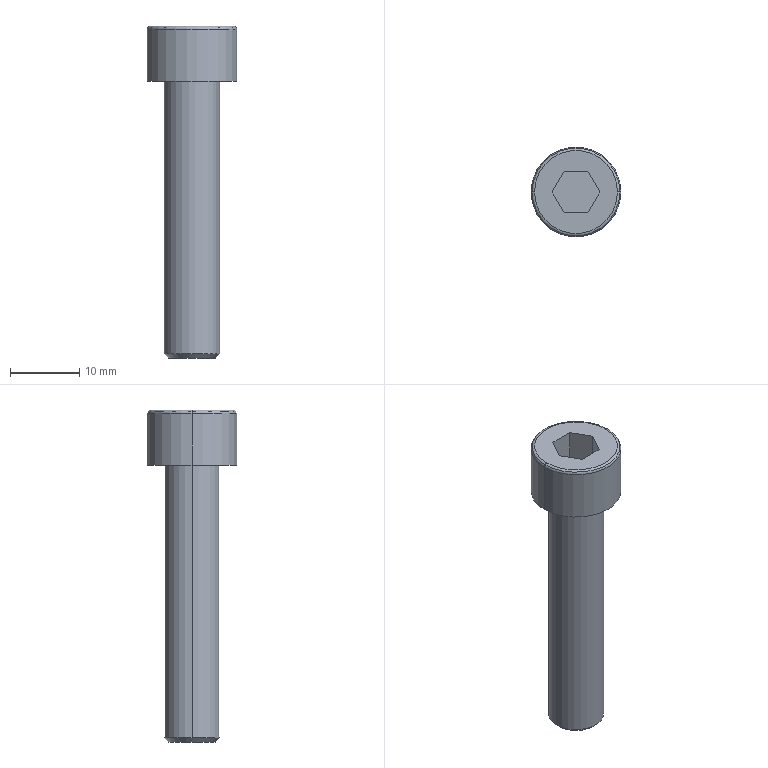Part | Creo | 1 solid | 20 faces | box 13 x 13 x 48 mm | volume 2901 mm3 | plane 10 | torus 4 | cylinder 4 | cone 2 | commonest cylinder face diameters 8 x2 13 x2
STEP:
#1=CARTESIAN_POINT('',(143.362,-96.002,37.161));
#2=VERTEX_POINT('',#1);
#3=CARTESIAN_POINT('',(131.362,-96.002,37.161));
#4=VERTEX_POINT('',#3);
#5=CARTESIAN_POINT('',(137.362,-96.002,37.161));
#6=DIRECTION('',(0.,0.,1.));
#7=DIRECTION('',(1.,0.,0.));
#8=AXIS2_PLACEMENT_3D('',#5,#6,#7);
#9=CIRCLE('',#8,6.);
#10=EDGE_CURVE('',#2,#4,#9,.T.);
#11=ORIENTED_EDGE('',*,*,#10,.F.);
#12=CARTESIAN_POINT('',(137.362,-96.002,37.161));
#13=DIRECTION('',(0.,0.,1.));
#14=DIRECTION('',(-1.,0.,0.));
#15=AXIS2_PLACEMENT_3D('',#12,#13,#14);
#16=CIRCLE('',#15,6.);
#17=EDGE_CURVE('',#4,#2,#16,.T.);
#18=ORIENTED_EDGE('',*,*,#17,.F.);
#19=EDGE_LOOP('',(#11,#18));
#20=FACE_OUTER_BOUND('',#19,.F.);
#21=CARTESIAN_POINT('',(139.094,-93.002,37.161));
#22=VERTEX_POINT('',#21);
#23=CARTESIAN_POINT('',(135.63,-93.002,37.161));
#24=VERTEX_POINT('',#23);
#25=CARTESIAN_POINT('',(139.094,-93.002,37.161));
#26=DIRECTION('',(-1.,0.,0.));
#27=VECTOR('',#26,3.464);
#28=LINE('',#25,#27);
#29=EDGE_CURVE('',#22,#24,#28,.T.);
#30=ORIENTED_EDGE('',*,*,#29,.T.);
#31=CARTESIAN_POINT('',(133.898,-96.002,37.161));
#32=VERTEX_POINT('',#31);
#33=CARTESIAN_POINT('',(133.898,-96.002,37.161));
#34=DIRECTION('',(0.5,0.866,0.));
#35=VECTOR('',#34,3.464);
#36=LINE('',#33,#35);
#37=EDGE_CURVE('',#32,#24,#36,.T.);
#38=ORIENTED_EDGE('',*,*,#37,.F.);
#39=CARTESIAN_POINT('',(135.63,-99.002,37.161));
#40=VERTEX_POINT('',#39);
#41=CARTESIAN_POINT('',(135.63,-99.002,37.161));
#42=DIRECTION('',(-0.5,0.866,0.));
#43=VECTOR('',#42,3.464);
#44=LINE('',#41,#43);
#45=EDGE_CURVE('',#40,#32,#44,.T.);
#46=ORIENTED_EDGE('',*,*,#45,.F.);
#47=CARTESIAN_POINT('',(139.094,-99.002,37.161));
#48=VERTEX_POINT('',#47);
#49=CARTESIAN_POINT('',(135.63,-99.002,37.161));
#50=DIRECTION('',(1.,0.,0.));
#51=VECTOR('',#50,3.464);
#52=LINE('',#49,#51);
#53=EDGE_CURVE('',#40,#48,#52,.T.);
#54=ORIENTED_EDGE('',*,*,#53,.T.);
#55=CARTESIAN_POINT('',(140.826,-96.002,37.161));
#56=VERTEX_POINT('',#55);
#57=CARTESIAN_POINT('',(140.826,-96.002,37.161));
#58=DIRECTION('',(-0.5,-0.866,0.));
#59=VECTOR('',#58,3.464);
#60=LINE('',#57,#59);
#61=EDGE_CURVE('',#56,#48,#60,.T.);
#62=ORIENTED_EDGE('',*,*,#61,.F.);
#63=CARTESIAN_POINT('',(139.094,-93.002,37.161));
#64=DIRECTION('',(0.5,-0.866,0.));
#65=VECTOR('',#64,3.464);
#66=LINE('',#63,#65);
#67=EDGE_CURVE('',#22,#56,#66,.T.);
#68=ORIENTED_EDGE('',*,*,#67,.F.);
#69=EDGE_LOOP('',(#30,#38,#46,#54,#62,#68));
#70=FACE_BOUND('',#69,.F.);
#71=CARTESIAN_POINT('',(137.362,-96.002,37.161));
#72=DIRECTION('',(0.,0.,1.));
#73=DIRECTION('',(1.,0.,0.));
#74=AXIS2_PLACEMENT_3D('',#71,#72,#73);
#75=PLANE('',#74);
#76=ADVANCED_FACE('',(#20,#70),#75,.T.);
#77=ORIENTED_EDGE('',*,*,#10,.T.);
#78=CARTESIAN_POINT('',(131.008,-96.002,37.014));
#79=VERTEX_POINT('',#78);
#80=CARTESIAN_POINT('',(131.362,-96.002,36.661));
#81=DIRECTION('',(0.,1.,0.));
#82=DIRECTION('',(-0.7071,0.,0.7071));
#83=AXIS2_PLACEMENT_3D('',#80,#81,#82);
#84=CIRCLE('',#83,0.5);
#85=EDGE_CURVE('',#79,#4,#84,.T.);
#86=ORIENTED_EDGE('',*,*,#85,.F.);
#87=CARTESIAN_POINT('',(143.715,-96.002,37.014));
#88=VERTEX_POINT('',#87);
#89=CARTESIAN_POINT('',(137.362,-96.002,37.014));
#90=DIRECTION('',(0.,0.,1.));
#91=DIRECTION('',(1.,0.,0.));
#92=AXIS2_PLACEMENT_3D('',#89,#90,#91);
#93=CIRCLE('',#92,6.354);
#94=EDGE_CURVE('',#88,#79,#93,.T.);
#95=ORIENTED_EDGE('',*,*,#94,.F.);
#96=CARTESIAN_POINT('',(143.362,-96.002,36.661));
#97=DIRECTION('',(0.,-1.,0.));
#98=DIRECTION('',(0.7071,0.,0.7071));
#99=AXIS2_PLACEMENT_3D('',#96,#97,#98);
#100=CIRCLE('',#99,0.5);
#101=EDGE_CURVE('',#88,#2,#100,.T.);
#102=ORIENTED_EDGE('',*,*,#101,.T.);
#103=EDGE_LOOP('',(#77,#86,#95,#102));
#104=FACE_OUTER_BOUND('',#103,.F.);
#105=CARTESIAN_POINT('',(137.362,-96.002,36.661));
#106=DIRECTION('',(0.,0.,1.));
#107=DIRECTION('',(1.,0.,0.));
#108=AXIS2_PLACEMENT_3D('',#105,#106,#107);
#109=TOROIDAL_SURFACE('',#108,6.,0.5);
#110=ADVANCED_FACE('',(#104),#109,.T.);
#111=ORIENTED_EDGE('',*,*,#17,.T.);
#112=ORIENTED_EDGE('',*,*,#101,.F.);
#113=CARTESIAN_POINT('',(137.362,-96.002,37.014));
#114=DIRECTION('',(0.,0.,1.));
#115=DIRECTION('',(-1.,0.,0.));
#116=AXIS2_PLACEMENT_3D('',#113,#114,#115);
#117=CIRCLE('',#116,6.354);
#118=EDGE_CURVE('',#79,#88,#117,.T.);
#119=ORIENTED_EDGE('',*,*,#118,.F.);
#120=ORIENTED_EDGE('',*,*,#85,.T.);
#121=EDGE_LOOP('',(#111,#112,#119,#120));
#122=FACE_OUTER_BOUND('',#121,.F.);
#123=CARTESIAN_POINT('',(137.362,-96.002,36.661));
#124=DIRECTION('',(0.,0.,1.));
#125=DIRECTION('',(1.,0.,0.));
#126=AXIS2_PLACEMENT_3D('',#123,#124,#125);
#127=TOROIDAL_SURFACE('',#126,6.,0.5);
#128=ADVANCED_FACE('',(#122),#127,.T.);
#129=CARTESIAN_POINT('',(130.862,-96.002,36.661));
#130=VERTEX_POINT('',#129);
#131=CARTESIAN_POINT('',(143.862,-96.002,36.661));
#132=VERTEX_POINT('',#131);
#133=CARTESIAN_POINT('',(137.362,-96.002,36.661));
#134=DIRECTION('',(0.,0.,1.));
#135=DIRECTION('',(-1.,0.,0.));
#136=AXIS2_PLACEMENT_3D('',#133,#134,#135);
#137=CIRCLE('',#136,6.5);
#138=EDGE_CURVE('',#130,#132,#137,.T.);
#139=ORIENTED_EDGE('',*,*,#138,.F.);
#140=CARTESIAN_POINT('',(131.362,-96.002,36.661));
#141=DIRECTION('',(0.,1.,0.));
#142=DIRECTION('',(-1.,0.,0.));
#143=AXIS2_PLACEMENT_3D('',#140,#141,#142);
#144=CIRCLE('',#143,0.5);
#145=EDGE_CURVE('',#130,#79,#144,.T.);
#146=ORIENTED_EDGE('',*,*,#145,.T.);
#147=ORIENTED_EDGE('',*,*,#118,.T.);
#148=CARTESIAN_POINT('',(143.362,-96.002,36.661));
#149=DIRECTION('',(0.,-1.,0.));
#150=DIRECTION('',(1.,0.,0.));
#151=AXIS2_PLACEMENT_3D('',#148,#149,#150);
#152=CIRCLE('',#151,0.5);
#153=EDGE_CURVE('',#132,#88,#152,.T.);
#154=ORIENTED_EDGE('',*,*,#153,.F.);
#155=EDGE_LOOP('',(#139,#146,#147,#154));
#156=FACE_OUTER_BOUND('',#155,.F.);
#157=CARTESIAN_POINT('',(137.362,-96.002,36.661));
#158=DIRECTION('',(0.,0.,1.));
#159=DIRECTION('',(1.,0.,0.));
#160=AXIS2_PLACEMENT_3D('',#157,#158,#159);
#161=TOROIDAL_SURFACE('',#160,6.,0.5);
#162=ADVANCED_FACE('',(#156),#161,.T.);
#163=ORIENTED_EDGE('',*,*,#138,.T.);
#164=CARTESIAN_POINT('',(143.862,-96.002,29.161));
#165=VERTEX_POINT('',#164);
#166=CARTESIAN_POINT('',(143.862,-96.002,29.161));
#167=DIRECTION('',(0.,0.,1.));
#168=VECTOR('',#167,7.5);
#169=LINE('',#166,#168);
#170=EDGE_CURVE('',#165,#132,#169,.T.);
#171=ORIENTED_EDGE('',*,*,#170,.F.);
#172=CARTESIAN_POINT('',(130.862,-96.002,29.161));
#173=VERTEX_POINT('',#172);
#174=CARTESIAN_POINT('',(137.362,-96.002,29.161));
#175=DIRECTION('',(0.,0.,-1.));
#176=DIRECTION('',(1.,0.,0.));
#177=AXIS2_PLACEMENT_3D('',#174,#175,#176);
#178=CIRCLE('',#177,6.5);
#179=EDGE_CURVE('',#165,#173,#178,.T.);
#180=ORIENTED_EDGE('',*,*,#179,.T.);
#181=CARTESIAN_POINT('',(130.862,-96.002,29.161));
#182=DIRECTION('',(0.,0.,1.));
#183=VECTOR('',#182,7.5);
#184=LINE('',#181,#183);
#185=EDGE_CURVE('',#173,#130,#184,.T.);
#186=ORIENTED_EDGE('',*,*,#185,.T.);
#187=EDGE_LOOP('',(#163,#171,#180,#186));
#188=FACE_OUTER_BOUND('',#187,.F.);
#189=CARTESIAN_POINT('',(137.362,-96.002,29.161));
#190=DIRECTION('',(0.,0.,1.));
#191=DIRECTION('',(1.,0.,0.));
#192=AXIS2_PLACEMENT_3D('',#189,#190,#191);
#193=CYLINDRICAL_SURFACE('',#192,6.5);
#194=ADVANCED_FACE('',(#188),#193,.T.);
#195=CARTESIAN_POINT('',(137.362,-96.002,36.661));
#196=DIRECTION('',(0.,0.,1.));
#197=DIRECTION('',(1.,0.,0.));
#198=AXIS2_PLACEMENT_3D('',#195,#196,#197);
#199=CIRCLE('',#198,6.5);
#200=EDGE_CURVE('',#132,#130,#199,.T.);
#201=ORIENTED_EDGE('',*,*,#200,.T.);
#202=ORIENTED_EDGE('',*,*,#185,.F.);
#203=CARTESIAN_POINT('',(137.362,-96.002,29.161));
#204=DIRECTION('',(0.,0.,-1.));
#205=DIRECTION('',(-1.,0.,0.));
#206=AXIS2_PLACEMENT_3D('',#203,#204,#205);
#207=CIRCLE('',#206,6.5);
#208=EDGE_CURVE('',#173,#165,#207,.T.);
#209=ORIENTED_EDGE('',*,*,#208,.T.);
#210=ORIENTED_EDGE('',*,*,#170,.T.);
#211=EDGE_LOOP('',(#201,#202,#209,#210));
#212=FACE_OUTER_BOUND('',#211,.F.);
#213=CARTESIAN_POINT('',(137.362,-96.002,29.161));
#214=DIRECTION('',(0.,0.,1.));
#215=DIRECTION('',(1.,0.,0.));
#216=AXIS2_PLACEMENT_3D('',#213,#214,#215);
#217=CYLINDRICAL_SURFACE('',#216,6.5);
#218=ADVANCED_FACE('',(#212),#217,.T.);
#219=ORIENTED_EDGE('',*,*,#200,.F.);
#220=ORIENTED_EDGE('',*,*,#153,.T.);
#221=ORIENTED_EDGE('',*,*,#94,.T.);
#222=ORIENTED_EDGE('',*,*,#145,.F.);
#223=EDGE_LOOP('',(#219,#220,#221,#222));
#224=FACE_OUTER_BOUND('',#223,.F.);
#225=CARTESIAN_POINT('',(137.362,-96.002,36.661));
#226=DIRECTION('',(0.,0.,1.));
#227=DIRECTION('',(1.,0.,0.));
#228=AXIS2_PLACEMENT_3D('',#225,#226,#227);
#229=TOROIDAL_SURFACE('',#228,6.,0.5);
#230=ADVANCED_FACE('',(#224),#229,.T.);
#231=ORIENTED_EDGE('',*,*,#179,.F.);
#232=ORIENTED_EDGE('',*,*,#208,.F.);
#233=EDGE_LOOP('',(#231,#232));
#234=FACE_OUTER_BOUND('',#233,.F.);
#235=CARTESIAN_POINT('',(141.362,-96.002,29.161));
#236=VERTEX_POINT('',#235);
#237=CARTESIAN_POINT('',(133.362,-96.002,29.161));
#238=VERTEX_POINT('',#237);
#239=CARTESIAN_POINT('',(137.362,-96.002,29.161));
#240=DIRECTION('',(0.,0.,1.));
#241=DIRECTION('',(1.,0.,0.));
#242=AXIS2_PLACEMENT_3D('',#239,#240,#241);
#243=CIRCLE('',#242,4.);
#244=EDGE_CURVE('',#236,#238,#243,.T.);
#245=ORIENTED_EDGE('',*,*,#244,.F.);
#246=CARTESIAN_POINT('',(137.362,-96.002,29.161));
#247=DIRECTION('',(0.,0.,1.));
#248=DIRECTION('',(-1.,0.,0.));
#249=AXIS2_PLACEMENT_3D('',#246,#247,#248);
#250=CIRCLE('',#249,4.);
#251=EDGE_CURVE('',#238,#236,#250,.T.);
#252=ORIENTED_EDGE('',*,*,#251,.F.);
#253=EDGE_LOOP('',(#245,#252));
#254=FACE_BOUND('',#253,.F.);
#255=CARTESIAN_POINT('',(137.362,-96.002,29.161));
#256=DIRECTION('',(0.,0.,-1.));
#257=DIRECTION('',(-1.,0.,0.));
#258=AXIS2_PLACEMENT_3D('',#255,#256,#257);
#259=PLANE('',#258);
#260=ADVANCED_FACE('',(#234,#254),#259,.T.);
#261=CARTESIAN_POINT('',(133.362,-96.002,-10.239));
#262=VERTEX_POINT('',#261);
#263=CARTESIAN_POINT('',(141.362,-96.002,-10.239));
#264=VERTEX_POINT('',#263);
#265=CARTESIAN_POINT('',(137.362,-96.002,-10.239));
#266=DIRECTION('',(0.,0.,-1.));
#267=DIRECTION('',(-1.,0.,0.));
#268=AXIS2_PLACEMENT_3D('',#265,#266,#267);
#269=CIRCLE('',#268,4.);
#270=EDGE_CURVE('',#262,#264,#269,.T.);
#271=ORIENTED_EDGE('',*,*,#270,.T.);
#272=CARTESIAN_POINT('',(141.362,-96.002,-10.239));
#273=DIRECTION('',(0.,0.,1.));
#274=VECTOR('',#273,39.4);
#275=LINE('',#272,#274);
#276=EDGE_CURVE('',#264,#236,#275,.T.);
#277=ORIENTED_EDGE('',*,*,#276,.T.);
#278=ORIENTED_EDGE('',*,*,#244,.T.);
#279=CARTESIAN_POINT('',(133.362,-96.002,-10.239));
#280=DIRECTION('',(0.,0.,1.));
#281=VECTOR('',#280,39.4);
#282=LINE('',#279,#281);
#283=EDGE_CURVE('',#262,#238,#282,.T.);
#284=ORIENTED_EDGE('',*,*,#283,.F.);
#285=EDGE_LOOP('',(#271,#277,#278,#284));
#286=FACE_OUTER_BOUND('',#285,.F.);
#287=CARTESIAN_POINT('',(137.362,-96.002,-10.839));
#288=DIRECTION('',(0.,0.,1.));
#289=DIRECTION('',(1.,0.,0.));
#290=AXIS2_PLACEMENT_3D('',#287,#288,#289);
#291=CYLINDRICAL_SURFACE('',#290,4.);
#292=ADVANCED_FACE('',(#286),#291,.T.);
#293=CARTESIAN_POINT('',(133.962,-96.002,-10.839));
#294=VERTEX_POINT('',#293);
#295=CARTESIAN_POINT('',(140.762,-96.002,-10.839));
#296=VERTEX_POINT('',#295);
#297=CARTESIAN_POINT('',(137.362,-96.002,-10.839));
#298=DIRECTION('',(0.,0.,-1.));
#299=DIRECTION('',(-1.,0.,0.));
#300=AXIS2_PLACEMENT_3D('',#297,#298,#299);
#301=CIRCLE('',#300,3.4);
#302=EDGE_CURVE('',#294,#296,#301,.T.);
#303=ORIENTED_EDGE('',*,*,#302,.T.);
#304=CARTESIAN_POINT('',(140.762,-96.002,-10.839));
#305=DIRECTION('',(0.7071,0.,0.7071));
#306=VECTOR('',#305,0.8485);
#307=LINE('',#304,#306);
#308=EDGE_CURVE('',#296,#264,#307,.T.);
#309=ORIENTED_EDGE('',*,*,#308,.T.);
#310=ORIENTED_EDGE('',*,*,#270,.F.);
#311=CARTESIAN_POINT('',(133.962,-96.002,-10.839));
#312=DIRECTION('',(-0.7071,0.,0.7071));
#313=VECTOR('',#312,0.8485);
#314=LINE('',#311,#313);
#315=EDGE_CURVE('',#294,#262,#314,.T.);
#316=ORIENTED_EDGE('',*,*,#315,.F.);
#317=EDGE_LOOP('',(#303,#309,#310,#316));
#318=FACE_OUTER_BOUND('',#317,.F.);
#319=CARTESIAN_POINT('',(137.362,-96.002,-10.539));
#320=DIRECTION('',(0.,0.,1.));
#321=DIRECTION('',(1.,0.,0.));
#322=AXIS2_PLACEMENT_3D('',#319,#320,#321);
#323=CONICAL_SURFACE('',#322,3.7,45.);
#324=ADVANCED_FACE('',(#318),#323,.T.);
#325=CARTESIAN_POINT('',(137.362,-96.002,-10.839));
#326=DIRECTION('',(0.,0.,-1.));
#327=DIRECTION('',(1.,0.,0.));
#328=AXIS2_PLACEMENT_3D('',#325,#326,#327);
#329=CIRCLE('',#328,3.4);
#330=EDGE_CURVE('',#296,#294,#329,.T.);
#331=ORIENTED_EDGE('',*,*,#330,.F.);
#332=ORIENTED_EDGE('',*,*,#302,.F.);
#333=EDGE_LOOP('',(#331,#332));
#334=FACE_OUTER_BOUND('',#333,.F.);
#335=CARTESIAN_POINT('',(137.362,-96.002,-10.839));
#336=DIRECTION('',(0.,0.,1.));
#337=DIRECTION('',(1.,0.,0.));
#338=AXIS2_PLACEMENT_3D('',#335,#336,#337);
#339=PLANE('',#338);
#340=ADVANCED_FACE('',(#334),#339,.F.);
#341=ORIENTED_EDGE('',*,*,#330,.T.);
#342=ORIENTED_EDGE('',*,*,#315,.T.);
#343=CARTESIAN_POINT('',(137.362,-96.002,-10.239));
#344=DIRECTION('',(0.,0.,-1.));
#345=DIRECTION('',(1.,0.,0.));
#346=AXIS2_PLACEMENT_3D('',#343,#344,#345);
#347=CIRCLE('',#346,4.);
#348=EDGE_CURVE('',#264,#262,#347,.T.);
#349=ORIENTED_EDGE('',*,*,#348,.F.);
#350=ORIENTED_EDGE('',*,*,#308,.F.);
#351=EDGE_LOOP('',(#341,#342,#349,#350));
#352=FACE_OUTER_BOUND('',#351,.F.);
#353=CARTESIAN_POINT('',(137.362,-96.002,-10.539));
#354=DIRECTION('',(0.,0.,1.));
#355=DIRECTION('',(1.,0.,0.));
#356=AXIS2_PLACEMENT_3D('',#353,#354,#355);
#357=CONICAL_SURFACE('',#356,3.7,45.);
#358=ADVANCED_FACE('',(#352),#357,.T.);
#359=ORIENTED_EDGE('',*,*,#348,.T.);
#360=ORIENTED_EDGE('',*,*,#283,.T.);
#361=ORIENTED_EDGE('',*,*,#251,.T.);
#362=ORIENTED_EDGE('',*,*,#276,.F.);
#363=EDGE_LOOP('',(#359,#360,#361,#362));
#364=FACE_OUTER_BOUND('',#363,.F.);
#365=CARTESIAN_POINT('',(137.362,-96.002,-10.839));
#366=DIRECTION('',(0.,0.,1.));
#367=DIRECTION('',(1.,0.,0.));
#368=AXIS2_PLACEMENT_3D('',#365,#366,#367);
#369=CYLINDRICAL_SURFACE('',#368,4.);
#370=ADVANCED_FACE('',(#364),#369,.T.);
#371=ORIENTED_EDGE('',*,*,#29,.F.);
#372=CARTESIAN_POINT('',(139.094,-93.002,31.881));
#373=VERTEX_POINT('',#372);
#374=CARTESIAN_POINT('',(139.094,-93.002,37.161));
#375=DIRECTION('',(0.,0.,-1.));
#376=VECTOR('',#375,5.28);
#377=LINE('',#374,#376);
#378=EDGE_CURVE('',#22,#373,#377,.T.);
#379=ORIENTED_EDGE('',*,*,#378,.T.);
#380=CARTESIAN_POINT('',(135.63,-93.002,31.881));
#381=VERTEX_POINT('',#380);
#382=CARTESIAN_POINT('',(139.094,-93.002,31.881));
#383=DIRECTION('',(-1.,0.,0.));
#384=VECTOR('',#383,3.464);
#385=LINE('',#382,#384);
#386=EDGE_CURVE('',#373,#381,#385,.T.);
#387=ORIENTED_EDGE('',*,*,#386,.T.);
#388=CARTESIAN_POINT('',(135.63,-93.002,37.161));
#389=DIRECTION('',(0.,0.,-1.));
#390=VECTOR('',#389,5.28);
#391=LINE('',#388,#390);
#392=EDGE_CURVE('',#24,#381,#391,.T.);
#393=ORIENTED_EDGE('',*,*,#392,.F.);
#394=EDGE_LOOP('',(#371,#379,#387,#393));
#395=FACE_OUTER_BOUND('',#394,.F.);
#396=CARTESIAN_POINT('',(135.63,-93.002,31.881));
#397=DIRECTION('',(0.,-1.,0.));
#398=DIRECTION('',(0.,0.,-1.));
#399=AXIS2_PLACEMENT_3D('',#396,#397,#398);
#400=PLANE('',#399);
#401=ADVANCED_FACE('',(#395),#400,.T.);
#402=ORIENTED_EDGE('',*,*,#67,.T.);
#403=CARTESIAN_POINT('',(140.826,-96.002,31.881));
#404=VERTEX_POINT('',#403);
#405=CARTESIAN_POINT('',(140.826,-96.002,37.161));
#406=DIRECTION('',(0.,0.,-1.));
#407=VECTOR('',#406,5.28);
#408=LINE('',#405,#407);
#409=EDGE_CURVE('',#56,#404,#408,.T.);
#410=ORIENTED_EDGE('',*,*,#409,.T.);
#411=CARTESIAN_POINT('',(140.826,-96.002,31.881));
#412=DIRECTION('',(-0.5,0.866,0.));
#413=VECTOR('',#412,3.464);
#414=LINE('',#411,#413);
#415=EDGE_CURVE('',#404,#373,#414,.T.);
#416=ORIENTED_EDGE('',*,*,#415,.T.);
#417=ORIENTED_EDGE('',*,*,#378,.F.);
#418=EDGE_LOOP('',(#402,#410,#416,#417));
#419=FACE_OUTER_BOUND('',#418,.F.);
#420=CARTESIAN_POINT('',(139.094,-93.002,31.881));
#421=DIRECTION('',(-0.866,-0.5,0.));
#422=DIRECTION('',(0.5,-0.866,0.));
#423=AXIS2_PLACEMENT_3D('',#420,#421,#422);
#424=PLANE('',#423);
#425=ADVANCED_FACE('',(#419),#424,.T.);
#426=ORIENTED_EDGE('',*,*,#61,.T.);
#427=CARTESIAN_POINT('',(139.094,-99.002,31.881));
#428=VERTEX_POINT('',#427);
#429=CARTESIAN_POINT('',(139.094,-99.002,37.161));
#430=DIRECTION('',(0.,0.,-1.));
#431=VECTOR('',#430,5.28);
#432=LINE('',#429,#431);
#433=EDGE_CURVE('',#48,#428,#432,.T.);
#434=ORIENTED_EDGE('',*,*,#433,.T.);
#435=CARTESIAN_POINT('',(139.094,-99.002,31.881));
#436=DIRECTION('',(0.5,0.866,0.));
#437=VECTOR('',#436,3.464);
#438=LINE('',#435,#437);
#439=EDGE_CURVE('',#428,#404,#438,.T.);
#440=ORIENTED_EDGE('',*,*,#439,.T.);
#441=ORIENTED_EDGE('',*,*,#409,.F.);
#442=EDGE_LOOP('',(#426,#434,#440,#441));
#443=FACE_OUTER_BOUND('',#442,.F.);
#444=CARTESIAN_POINT('',(140.826,-96.002,31.881));
#445=DIRECTION('',(-0.866,0.5,0.));
#446=DIRECTION('',(-0.5,-0.866,0.));
#447=AXIS2_PLACEMENT_3D('',#444,#445,#446);
#448=PLANE('',#447);
#449=ADVANCED_FACE('',(#443),#448,.T.);
#450=ORIENTED_EDGE('',*,*,#53,.F.);
#451=CARTESIAN_POINT('',(135.63,-99.002,31.881));
#452=VERTEX_POINT('',#451);
#453=CARTESIAN_POINT('',(135.63,-99.002,37.161));
#454=DIRECTION('',(0.,0.,-1.));
#455=VECTOR('',#454,5.28);
#456=LINE('',#453,#455);
#457=EDGE_CURVE('',#40,#452,#456,.T.);
#458=ORIENTED_EDGE('',*,*,#457,.T.);
#459=CARTESIAN_POINT('',(135.63,-99.002,31.881));
#460=DIRECTION('',(1.,0.,0.));
#461=VECTOR('',#460,3.464);
#462=LINE('',#459,#461);
#463=EDGE_CURVE('',#452,#428,#462,.T.);
#464=ORIENTED_EDGE('',*,*,#463,.T.);
#465=ORIENTED_EDGE('',*,*,#433,.F.);
#466=EDGE_LOOP('',(#450,#458,#464,#465));
#467=FACE_OUTER_BOUND('',#466,.F.);
#468=CARTESIAN_POINT('',(139.094,-99.002,31.881));
#469=DIRECTION('',(0.,1.,0.));
#470=DIRECTION('',(0.,0.,1.));
#471=AXIS2_PLACEMENT_3D('',#468,#469,#470);
#472=PLANE('',#471);
#473=ADVANCED_FACE('',(#467),#472,.T.);
#474=ORIENTED_EDGE('',*,*,#45,.T.);
#475=CARTESIAN_POINT('',(133.898,-96.002,31.881));
#476=VERTEX_POINT('',#475);
#477=CARTESIAN_POINT('',(133.898,-96.002,37.161));
#478=DIRECTION('',(0.,0.,-1.));
#479=VECTOR('',#478,5.28);
#480=LINE('',#477,#479);
#481=EDGE_CURVE('',#32,#476,#480,.T.);
#482=ORIENTED_EDGE('',*,*,#481,.T.);
#483=CARTESIAN_POINT('',(133.898,-96.002,31.881));
#484=DIRECTION('',(0.5,-0.866,0.));
#485=VECTOR('',#484,3.464);
#486=LINE('',#483,#485);
#487=EDGE_CURVE('',#476,#452,#486,.T.);
#488=ORIENTED_EDGE('',*,*,#487,.T.);
#489=ORIENTED_EDGE('',*,*,#457,.F.);
#490=EDGE_LOOP('',(#474,#482,#488,#489));
#491=FACE_OUTER_BOUND('',#490,.F.);
#492=CARTESIAN_POINT('',(135.63,-99.002,31.881));
#493=DIRECTION('',(0.866,0.5,0.));
#494=DIRECTION('',(-0.5,0.866,0.));
#495=AXIS2_PLACEMENT_3D('',#492,#493,#494);
#496=PLANE('',#495);
#497=ADVANCED_FACE('',(#491),#496,.T.);
#498=ORIENTED_EDGE('',*,*,#37,.T.);
#499=ORIENTED_EDGE('',*,*,#392,.T.);
#500=CARTESIAN_POINT('',(135.63,-93.002,31.881));
#501=DIRECTION('',(-0.5,-0.866,0.));
#502=VECTOR('',#501,3.464);
#503=LINE('',#500,#502);
#504=EDGE_CURVE('',#381,#476,#503,.T.);
#505=ORIENTED_EDGE('',*,*,#504,.T.);
#506=ORIENTED_EDGE('',*,*,#481,.F.);
#507=EDGE_LOOP('',(#498,#499,#505,#506));
#508=FACE_OUTER_BOUND('',#507,.F.);
#509=CARTESIAN_POINT('',(133.898,-96.002,31.881));
#510=DIRECTION('',(0.866,-0.5,0.));
#511=DIRECTION('',(0.5,0.866,0.));
#512=AXIS2_PLACEMENT_3D('',#509,#510,#511);
#513=PLANE('',#512);
#514=ADVANCED_FACE('',(#508),#513,.T.);
#515=ORIENTED_EDGE('',*,*,#415,.F.);
#516=ORIENTED_EDGE('',*,*,#439,.F.);
#517=ORIENTED_EDGE('',*,*,#463,.F.);
#518=ORIENTED_EDGE('',*,*,#487,.F.);
#519=ORIENTED_EDGE('',*,*,#504,.F.);
#520=ORIENTED_EDGE('',*,*,#386,.F.);
#521=EDGE_LOOP('',(#515,#516,#517,#518,#519,#520));
#522=FACE_OUTER_BOUND('',#521,.F.);
#523=CARTESIAN_POINT('',(142.558,-99.002,31.881));
#524=DIRECTION('',(0.,0.,-1.));
#525=DIRECTION('',(-1.,0.,0.));
#526=AXIS2_PLACEMENT_3D('',#523,#524,#525);
#527=PLANE('',#526);
#528=ADVANCED_FACE('',(#522),#527,.F.);
#529=CLOSED_SHELL('',(#76,#110,#128,#162,#194,#218,#230,#260,#292,#324,#340,#358,#370,#401,#425,#449,#473,#497,#514,#528));
#530=MANIFOLD_SOLID_BREP('',#529);
#531=(LENGTH_UNIT()NAMED_UNIT(*)SI_UNIT(.MILLI.,.METRE.));
#532=UNCERTAINTY_MEASURE_WITH_UNIT(LENGTH_MEASURE(0.00514),#531,'','');
#533=(NAMED_UNIT(*)PLANE_ANGLE_UNIT()SI_UNIT($,.RADIAN.));
#534=PLANE_ANGLE_MEASURE_WITH_UNIT(PLANE_ANGLE_MEASURE(0.01745),#533);
#535=(CONVERSION_BASED_UNIT('DEGREE',#534)NAMED_UNIT(*)PLANE_ANGLE_UNIT());
#536=(NAMED_UNIT(*)SI_UNIT($,.STERADIAN.)SOLID_ANGLE_UNIT());
#537=(GEOMETRIC_REPRESENTATION_CONTEXT(3)GLOBAL_UNCERTAINTY_ASSIGNED_CONTEXT((#532))GLOBAL_UNIT_ASSIGNED_CONTEXT((#531,#535,#536))REPRESENTATION_CONTEXT('',''));
#538=ADVANCED_BREP_SHAPE_REPRESENTATION('',(#530),#537);